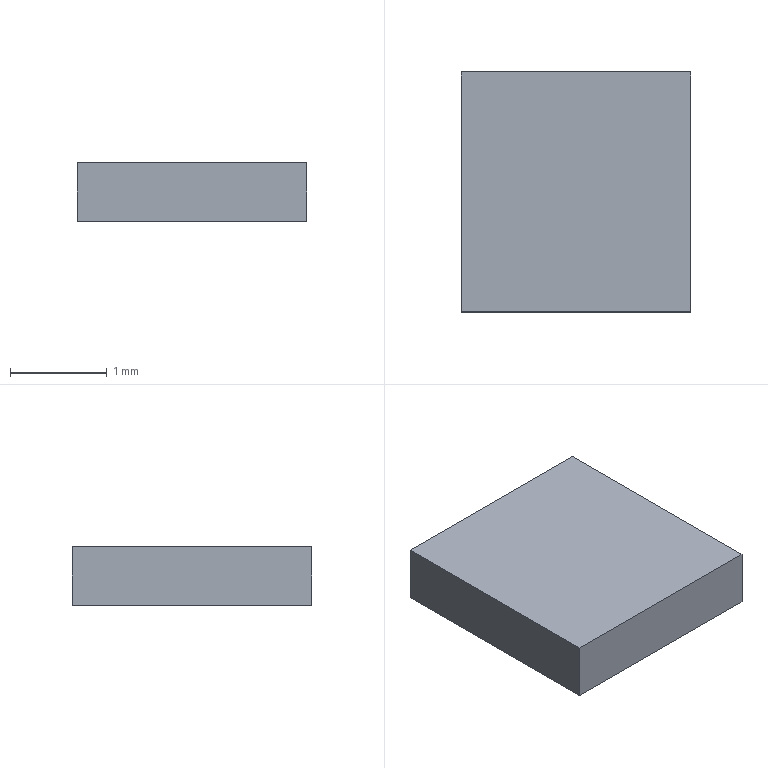Part | Creo | 1 solid | 6 faces | box 2.368 x 2.475 x 0.6 mm | volume 3.517 mm3 | plane 6
STEP:
#1=CARTESIAN_POINT('',(0.,0.,0.));
#2=DIRECTION('',(0.,0.,1.));
#3=DIRECTION('',(1.,0.,0.));
#4=AXIS2_PLACEMENT_3D('',#1,#2,#3);
#5=CARTESIAN_POINT('',(-1.218,-1.325,0.));
#6=VERTEX_POINT('',#5);
#7=CARTESIAN_POINT('',(1.15,-1.325,0.));
#8=VERTEX_POINT('',#7);
#9=CARTESIAN_POINT('',(-1.218,-1.325,0.));
#10=DIRECTION('',(1.,0.,0.));
#11=VECTOR('',#10,2.368);
#12=LINE('',#9,#11);
#13=EDGE_CURVE('',#6,#8,#12,.T.);
#14=ORIENTED_EDGE('',*,*,#13,.T.);
#15=CARTESIAN_POINT('',(1.15,1.15,0.));
#16=VERTEX_POINT('',#15);
#17=CARTESIAN_POINT('',(1.15,-1.325,0.));
#18=DIRECTION('',(0.,1.,0.));
#19=VECTOR('',#18,2.475);
#20=LINE('',#17,#19);
#21=EDGE_CURVE('',#8,#16,#20,.T.);
#22=ORIENTED_EDGE('',*,*,#21,.T.);
#23=CARTESIAN_POINT('',(-1.218,1.15,0.));
#24=VERTEX_POINT('',#23);
#25=CARTESIAN_POINT('',(1.15,1.15,0.));
#26=DIRECTION('',(-1.,0.,0.));
#27=VECTOR('',#26,2.368);
#28=LINE('',#25,#27);
#29=EDGE_CURVE('',#16,#24,#28,.T.);
#30=ORIENTED_EDGE('',*,*,#29,.T.);
#31=CARTESIAN_POINT('',(-1.218,1.15,0.));
#32=DIRECTION('',(0.,-1.,0.));
#33=VECTOR('',#32,2.475);
#34=LINE('',#31,#33);
#35=EDGE_CURVE('',#24,#6,#34,.T.);
#36=ORIENTED_EDGE('',*,*,#35,.T.);
#37=EDGE_LOOP('',(#14,#22,#30,#36));
#38=FACE_OUTER_BOUND('',#37,.F.);
#39=CARTESIAN_POINT('',(0.,0.,0.));
#40=DIRECTION('',(0.,0.,1.));
#41=DIRECTION('',(1.,0.,0.));
#42=AXIS2_PLACEMENT_3D('',#39,#40,#41);
#43=PLANE('',#42);
#44=ADVANCED_FACE('',(#38),#43,.F.);
#45=ORIENTED_EDGE('',*,*,#13,.F.);
#46=CARTESIAN_POINT('',(-1.218,-1.325,0.6));
#47=VERTEX_POINT('',#46);
#48=CARTESIAN_POINT('',(-1.218,-1.325,0.));
#49=DIRECTION('',(0.,0.,1.));
#50=VECTOR('',#49,0.6);
#51=LINE('',#48,#50);
#52=EDGE_CURVE('',#6,#47,#51,.T.);
#53=ORIENTED_EDGE('',*,*,#52,.T.);
#54=CARTESIAN_POINT('',(1.15,-1.325,0.6));
#55=VERTEX_POINT('',#54);
#56=CARTESIAN_POINT('',(-1.218,-1.325,0.6));
#57=DIRECTION('',(1.,0.,0.));
#58=VECTOR('',#57,2.368);
#59=LINE('',#56,#58);
#60=EDGE_CURVE('',#47,#55,#59,.T.);
#61=ORIENTED_EDGE('',*,*,#60,.T.);
#62=CARTESIAN_POINT('',(1.15,-1.325,0.));
#63=DIRECTION('',(0.,0.,1.));
#64=VECTOR('',#63,0.6);
#65=LINE('',#62,#64);
#66=EDGE_CURVE('',#8,#55,#65,.T.);
#67=ORIENTED_EDGE('',*,*,#66,.F.);
#68=EDGE_LOOP('',(#45,#53,#61,#67));
#69=FACE_OUTER_BOUND('',#68,.F.);
#70=CARTESIAN_POINT('',(-1.218,-1.325,0.));
#71=DIRECTION('',(0.,-1.,0.));
#72=DIRECTION('',(1.,0.,0.));
#73=AXIS2_PLACEMENT_3D('',#70,#71,#72);
#74=PLANE('',#73);
#75=ADVANCED_FACE('',(#69),#74,.T.);
#76=ORIENTED_EDGE('',*,*,#35,.F.);
#77=CARTESIAN_POINT('',(-1.218,1.15,0.6));
#78=VERTEX_POINT('',#77);
#79=CARTESIAN_POINT('',(-1.218,1.15,0.));
#80=DIRECTION('',(0.,0.,1.));
#81=VECTOR('',#80,0.6);
#82=LINE('',#79,#81);
#83=EDGE_CURVE('',#24,#78,#82,.T.);
#84=ORIENTED_EDGE('',*,*,#83,.T.);
#85=CARTESIAN_POINT('',(-1.218,1.15,0.6));
#86=DIRECTION('',(0.,-1.,0.));
#87=VECTOR('',#86,2.475);
#88=LINE('',#85,#87);
#89=EDGE_CURVE('',#78,#47,#88,.T.);
#90=ORIENTED_EDGE('',*,*,#89,.T.);
#91=ORIENTED_EDGE('',*,*,#52,.F.);
#92=EDGE_LOOP('',(#76,#84,#90,#91));
#93=FACE_OUTER_BOUND('',#92,.F.);
#94=CARTESIAN_POINT('',(-1.218,1.15,0.));
#95=DIRECTION('',(-1.,0.,0.));
#96=DIRECTION('',(0.,-1.,0.));
#97=AXIS2_PLACEMENT_3D('',#94,#95,#96);
#98=PLANE('',#97);
#99=ADVANCED_FACE('',(#93),#98,.T.);
#100=ORIENTED_EDGE('',*,*,#29,.F.);
#101=CARTESIAN_POINT('',(1.15,1.15,0.6));
#102=VERTEX_POINT('',#101);
#103=CARTESIAN_POINT('',(1.15,1.15,0.));
#104=DIRECTION('',(0.,0.,1.));
#105=VECTOR('',#104,0.6);
#106=LINE('',#103,#105);
#107=EDGE_CURVE('',#16,#102,#106,.T.);
#108=ORIENTED_EDGE('',*,*,#107,.T.);
#109=CARTESIAN_POINT('',(1.15,1.15,0.6));
#110=DIRECTION('',(-1.,0.,0.));
#111=VECTOR('',#110,2.368);
#112=LINE('',#109,#111);
#113=EDGE_CURVE('',#102,#78,#112,.T.);
#114=ORIENTED_EDGE('',*,*,#113,.T.);
#115=ORIENTED_EDGE('',*,*,#83,.F.);
#116=EDGE_LOOP('',(#100,#108,#114,#115));
#117=FACE_OUTER_BOUND('',#116,.F.);
#118=CARTESIAN_POINT('',(1.15,1.15,0.));
#119=DIRECTION('',(0.,1.,0.));
#120=DIRECTION('',(-1.,0.,0.));
#121=AXIS2_PLACEMENT_3D('',#118,#119,#120);
#122=PLANE('',#121);
#123=ADVANCED_FACE('',(#117),#122,.T.);
#124=ORIENTED_EDGE('',*,*,#21,.F.);
#125=ORIENTED_EDGE('',*,*,#66,.T.);
#126=CARTESIAN_POINT('',(1.15,-1.325,0.6));
#127=DIRECTION('',(0.,1.,0.));
#128=VECTOR('',#127,2.475);
#129=LINE('',#126,#128);
#130=EDGE_CURVE('',#55,#102,#129,.T.);
#131=ORIENTED_EDGE('',*,*,#130,.T.);
#132=ORIENTED_EDGE('',*,*,#107,.F.);
#133=EDGE_LOOP('',(#124,#125,#131,#132));
#134=FACE_OUTER_BOUND('',#133,.F.);
#135=CARTESIAN_POINT('',(1.15,-1.325,0.));
#136=DIRECTION('',(1.,0.,0.));
#137=DIRECTION('',(0.,1.,0.));
#138=AXIS2_PLACEMENT_3D('',#135,#136,#137);
#139=PLANE('',#138);
#140=ADVANCED_FACE('',(#134),#139,.T.);
#141=ORIENTED_EDGE('',*,*,#60,.F.);
#142=ORIENTED_EDGE('',*,*,#89,.F.);
#143=ORIENTED_EDGE('',*,*,#113,.F.);
#144=ORIENTED_EDGE('',*,*,#130,.F.);
#145=EDGE_LOOP('',(#141,#142,#143,#144));
#146=FACE_OUTER_BOUND('',#145,.F.);
#147=CARTESIAN_POINT('',(0.,0.,0.6));
#148=DIRECTION('',(0.,0.,1.));
#149=DIRECTION('',(1.,0.,0.));
#150=AXIS2_PLACEMENT_3D('',#147,#148,#149);
#151=PLANE('',#150);
#152=ADVANCED_FACE('',(#146),#151,.T.);
#153=CLOSED_SHELL('',(#44,#75,#99,#123,#140,#152));
#154=MANIFOLD_SOLID_BREP('',#153);
#155=(LENGTH_UNIT()NAMED_UNIT(*)SI_UNIT(.MILLI.,.METRE.));
#156=UNCERTAINTY_MEASURE_WITH_UNIT(LENGTH_MEASURE(0.0003478),#155,'','');
#157=(NAMED_UNIT(*)PLANE_ANGLE_UNIT()SI_UNIT($,.RADIAN.));
#158=PLANE_ANGLE_MEASURE_WITH_UNIT(PLANE_ANGLE_MEASURE(0.01745),#157);
#159=(CONVERSION_BASED_UNIT('DEGREE',#158)NAMED_UNIT(*)PLANE_ANGLE_UNIT());
#160=(NAMED_UNIT(*)SI_UNIT($,.STERADIAN.)SOLID_ANGLE_UNIT());
#161=(GEOMETRIC_REPRESENTATION_CONTEXT(3)GLOBAL_UNCERTAINTY_ASSIGNED_CONTEXT((#156))GLOBAL_UNIT_ASSIGNED_CONTEXT((#155,#159,#160))REPRESENTATION_CONTEXT('',''));
#162=ADVANCED_BREP_SHAPE_REPRESENTATION('',(#4,#154),#161);